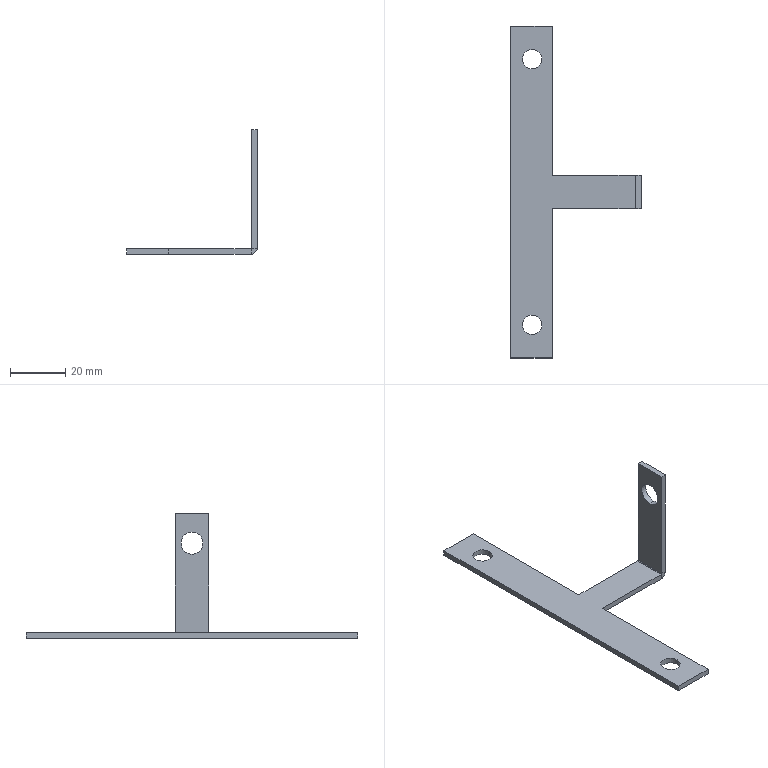Part | STEP file | Sensor bracket | 1 solid | 24 faces | box 47.2 x 120 x 45 mm | volume 5138 mm3 | plane 16 | cylinder 8 | commonest cylinder face diameters 7 x4 8 x2 0.4 x1 4.4 x1
STEP:
#1=CARTESIAN_POINT('',(39.7,0.,36.373));
#2=VERTEX_POINT('',#1);
#3=CARTESIAN_POINT('',(39.7,0.,28.373));
#4=VERTEX_POINT('',#3);
#5=CARTESIAN_POINT('',(39.7,0.,32.373));
#6=DIRECTION('',(1.,0.,0.));
#7=DIRECTION('',(0.,0.,1.));
#8=AXIS2_PLACEMENT_3D('',#5,#6,#7);
#9=CIRCLE('',#8,4.);
#10=EDGE_CURVE('',#2,#4,#9,.T.);
#11=ORIENTED_EDGE('',*,*,#10,.T.);
#12=CARTESIAN_POINT('',(37.7,0.,28.373));
#13=VERTEX_POINT('',#12);
#14=CARTESIAN_POINT('',(39.701,0.,28.373));
#15=DIRECTION('',(-1.,0.,0.));
#16=VECTOR('',#15,1000.);
#17=LINE('',#14,#16);
#18=EDGE_CURVE('',#4,#13,#17,.T.);
#19=ORIENTED_EDGE('',*,*,#18,.T.);
#20=CARTESIAN_POINT('',(37.7,0.,36.373));
#21=VERTEX_POINT('',#20);
#22=CARTESIAN_POINT('',(37.7,0.,32.373));
#23=DIRECTION('',(-1.,0.,0.));
#24=DIRECTION('',(0.,0.,1.));
#25=AXIS2_PLACEMENT_3D('',#22,#23,#24);
#26=CIRCLE('',#25,4.);
#27=EDGE_CURVE('',#13,#21,#26,.T.);
#28=ORIENTED_EDGE('',*,*,#27,.T.);
#29=CARTESIAN_POINT('',(39.701,0.,36.373));
#30=DIRECTION('',(-1.,0.,0.));
#31=VECTOR('',#30,1000.);
#32=LINE('',#29,#31);
#33=EDGE_CURVE('',#2,#21,#32,.T.);
#34=ORIENTED_EDGE('',*,*,#33,.F.);
#35=EDGE_LOOP('',(#11,#19,#28,#34));
#36=FACE_OUTER_BOUND('',#35,.T.);
#37=CARTESIAN_POINT('',(39.701,0.,32.373));
#38=DIRECTION('',(-1.,0.,0.));
#39=DIRECTION('',(0.,0.,1.));
#40=AXIS2_PLACEMENT_3D('',#37,#38,#39);
#41=CYLINDRICAL_SURFACE('',#40,4.);
#42=ADVANCED_FACE('',(#36),#41,.F.);
#43=CARTESIAN_POINT('',(-3.236,48.,-2.));
#44=VERTEX_POINT('',#43);
#45=CARTESIAN_POINT('',(3.764,48.,-2.));
#46=VERTEX_POINT('',#45);
#47=CARTESIAN_POINT('',(0.2639,48.,-2.));
#48=DIRECTION('',(0.,0.,1.));
#49=DIRECTION('',(-1.,0.,0.));
#50=AXIS2_PLACEMENT_3D('',#47,#48,#49);
#51=CIRCLE('',#50,3.5);
#52=EDGE_CURVE('',#44,#46,#51,.T.);
#53=ORIENTED_EDGE('',*,*,#52,.F.);
#54=CARTESIAN_POINT('',(-3.236,48.,0.));
#55=VERTEX_POINT('',#54);
#56=CARTESIAN_POINT('',(-3.236,48.,-2.001));
#57=DIRECTION('',(0.,0.,1.));
#58=VECTOR('',#57,1000.);
#59=LINE('',#56,#58);
#60=EDGE_CURVE('',#44,#55,#59,.T.);
#61=ORIENTED_EDGE('',*,*,#60,.T.);
#62=CARTESIAN_POINT('',(3.764,48.,0.));
#63=VERTEX_POINT('',#62);
#64=CARTESIAN_POINT('',(0.2639,48.,0.));
#65=DIRECTION('',(0.,0.,1.));
#66=DIRECTION('',(1.,0.,0.));
#67=AXIS2_PLACEMENT_3D('',#64,#65,#66);
#68=CIRCLE('',#67,3.5);
#69=EDGE_CURVE('',#55,#63,#68,.T.);
#70=ORIENTED_EDGE('',*,*,#69,.T.);
#71=CARTESIAN_POINT('',(3.764,48.,-2.001));
#72=DIRECTION('',(0.,0.,1.));
#73=VECTOR('',#72,1000.);
#74=LINE('',#71,#73);
#75=EDGE_CURVE('',#46,#63,#74,.T.);
#76=ORIENTED_EDGE('',*,*,#75,.F.);
#77=EDGE_LOOP('',(#53,#61,#70,#76));
#78=FACE_OUTER_BOUND('',#77,.T.);
#79=CARTESIAN_POINT('',(0.2639,48.,-2.001));
#80=DIRECTION('',(0.,0.,1.));
#81=DIRECTION('',(1.,0.,0.));
#82=AXIS2_PLACEMENT_3D('',#79,#80,#81);
#83=CYLINDRICAL_SURFACE('',#82,3.5);
#84=ADVANCED_FACE('',(#78),#83,.F.);
#85=CARTESIAN_POINT('',(-3.236,-48.,-2.));
#86=VERTEX_POINT('',#85);
#87=CARTESIAN_POINT('',(3.764,-48.,-2.));
#88=VERTEX_POINT('',#87);
#89=CARTESIAN_POINT('',(0.2639,-48.,-2.));
#90=DIRECTION('',(0.,0.,1.));
#91=DIRECTION('',(-1.,0.,0.));
#92=AXIS2_PLACEMENT_3D('',#89,#90,#91);
#93=CIRCLE('',#92,3.5);
#94=EDGE_CURVE('',#86,#88,#93,.T.);
#95=ORIENTED_EDGE('',*,*,#94,.F.);
#96=CARTESIAN_POINT('',(-3.236,-48.,0.));
#97=VERTEX_POINT('',#96);
#98=CARTESIAN_POINT('',(-3.236,-48.,-2.001));
#99=DIRECTION('',(0.,0.,1.));
#100=VECTOR('',#99,1000.);
#101=LINE('',#98,#100);
#102=EDGE_CURVE('',#86,#97,#101,.T.);
#103=ORIENTED_EDGE('',*,*,#102,.T.);
#104=CARTESIAN_POINT('',(3.764,-48.,0.));
#105=VERTEX_POINT('',#104);
#106=CARTESIAN_POINT('',(0.2639,-48.,0.));
#107=DIRECTION('',(0.,0.,1.));
#108=DIRECTION('',(1.,0.,0.));
#109=AXIS2_PLACEMENT_3D('',#106,#107,#108);
#110=CIRCLE('',#109,3.5);
#111=EDGE_CURVE('',#97,#105,#110,.T.);
#112=ORIENTED_EDGE('',*,*,#111,.T.);
#113=CARTESIAN_POINT('',(3.764,-48.,-2.001));
#114=DIRECTION('',(0.,0.,1.));
#115=VECTOR('',#114,1000.);
#116=LINE('',#113,#115);
#117=EDGE_CURVE('',#88,#105,#116,.T.);
#118=ORIENTED_EDGE('',*,*,#117,.F.);
#119=EDGE_LOOP('',(#95,#103,#112,#118));
#120=FACE_OUTER_BOUND('',#119,.T.);
#121=CARTESIAN_POINT('',(0.2639,-48.,-2.001));
#122=DIRECTION('',(0.,0.,1.));
#123=DIRECTION('',(1.,0.,0.));
#124=AXIS2_PLACEMENT_3D('',#121,#122,#123);
#125=CYLINDRICAL_SURFACE('',#124,3.5);
#126=ADVANCED_FACE('',(#120),#125,.F.);
#127=CARTESIAN_POINT('',(7.5,6.,0.));
#128=VERTEX_POINT('',#127);
#129=CARTESIAN_POINT('',(7.5,60.,0.));
#130=VERTEX_POINT('',#129);
#131=CARTESIAN_POINT('',(7.5,6.,0.));
#132=DIRECTION('',(0.,1.,0.));
#133=VECTOR('',#132,1000.);
#134=LINE('',#131,#133);
#135=EDGE_CURVE('',#128,#130,#134,.T.);
#136=ORIENTED_EDGE('',*,*,#135,.F.);
#137=CARTESIAN_POINT('',(7.5,6.,-2.));
#138=VERTEX_POINT('',#137);
#139=CARTESIAN_POINT('',(7.5,6.,-2.));
#140=DIRECTION('',(0.,0.,1.));
#141=VECTOR('',#140,1000.);
#142=LINE('',#139,#141);
#143=EDGE_CURVE('',#138,#128,#142,.T.);
#144=ORIENTED_EDGE('',*,*,#143,.F.);
#145=CARTESIAN_POINT('',(7.5,60.,-2.));
#146=VERTEX_POINT('',#145);
#147=CARTESIAN_POINT('',(7.5,6.,-2.));
#148=DIRECTION('',(0.,1.,0.));
#149=VECTOR('',#148,1000.);
#150=LINE('',#147,#149);
#151=EDGE_CURVE('',#138,#146,#150,.T.);
#152=ORIENTED_EDGE('',*,*,#151,.T.);
#153=CARTESIAN_POINT('',(7.5,60.,-2.));
#154=DIRECTION('',(0.,0.,1.));
#155=VECTOR('',#154,1000.);
#156=LINE('',#153,#155);
#157=EDGE_CURVE('',#146,#130,#156,.T.);
#158=ORIENTED_EDGE('',*,*,#157,.T.);
#159=EDGE_LOOP('',(#136,#144,#152,#158));
#160=FACE_OUTER_BOUND('',#159,.T.);
#161=CARTESIAN_POINT('',(7.5,6.,-2.));
#162=DIRECTION('',(1.,0.,0.));
#163=DIRECTION('',(0.,1.,0.));
#164=AXIS2_PLACEMENT_3D('',#161,#162,#163);
#165=PLANE('',#164);
#166=ADVANCED_FACE('',(#160),#165,.T.);
#167=CARTESIAN_POINT('',(37.5,6.,0.));
#168=VERTEX_POINT('',#167);
#169=CARTESIAN_POINT('',(37.5,6.,0.));
#170=DIRECTION('',(-1.,0.,0.));
#171=VECTOR('',#170,1000.);
#172=LINE('',#169,#171);
#173=EDGE_CURVE('',#168,#128,#172,.T.);
#174=ORIENTED_EDGE('',*,*,#173,.F.);
#175=CARTESIAN_POINT('',(37.5,6.,-2.));
#176=VERTEX_POINT('',#175);
#177=CARTESIAN_POINT('',(37.5,6.,-2.));
#178=DIRECTION('',(0.,0.,1.));
#179=VECTOR('',#178,1000.);
#180=LINE('',#177,#179);
#181=EDGE_CURVE('',#176,#168,#180,.T.);
#182=ORIENTED_EDGE('',*,*,#181,.F.);
#183=CARTESIAN_POINT('',(37.5,6.,-2.));
#184=DIRECTION('',(-1.,0.,0.));
#185=VECTOR('',#184,1000.);
#186=LINE('',#183,#185);
#187=EDGE_CURVE('',#176,#138,#186,.T.);
#188=ORIENTED_EDGE('',*,*,#187,.T.);
#189=ORIENTED_EDGE('',*,*,#143,.T.);
#190=EDGE_LOOP('',(#174,#182,#188,#189));
#191=FACE_OUTER_BOUND('',#190,.T.);
#192=CARTESIAN_POINT('',(37.5,6.,-2.));
#193=DIRECTION('',(0.,1.,0.));
#194=DIRECTION('',(-1.,0.,0.));
#195=AXIS2_PLACEMENT_3D('',#192,#193,#194);
#196=PLANE('',#195);
#197=ADVANCED_FACE('',(#191),#196,.T.);
#198=CARTESIAN_POINT('',(7.5,-6.,0.));
#199=VERTEX_POINT('',#198);
#200=CARTESIAN_POINT('',(37.5,-6.,0.));
#201=VERTEX_POINT('',#200);
#202=CARTESIAN_POINT('',(37.5,-6.,0.));
#203=DIRECTION('',(1.,0.,0.));
#204=VECTOR('',#203,1000.);
#205=LINE('',#202,#204);
#206=EDGE_CURVE('',#199,#201,#205,.T.);
#207=ORIENTED_EDGE('',*,*,#206,.F.);
#208=CARTESIAN_POINT('',(7.5,-6.,-2.));
#209=VERTEX_POINT('',#208);
#210=CARTESIAN_POINT('',(7.5,-6.,-2.));
#211=DIRECTION('',(0.,0.,1.));
#212=VECTOR('',#211,1000.);
#213=LINE('',#210,#212);
#214=EDGE_CURVE('',#209,#199,#213,.T.);
#215=ORIENTED_EDGE('',*,*,#214,.F.);
#216=CARTESIAN_POINT('',(37.5,-6.,-2.));
#217=VERTEX_POINT('',#216);
#218=CARTESIAN_POINT('',(37.5,-6.,-2.));
#219=DIRECTION('',(1.,0.,0.));
#220=VECTOR('',#219,1000.);
#221=LINE('',#218,#220);
#222=EDGE_CURVE('',#209,#217,#221,.T.);
#223=ORIENTED_EDGE('',*,*,#222,.T.);
#224=CARTESIAN_POINT('',(37.5,-6.,-2.));
#225=DIRECTION('',(0.,0.,1.));
#226=VECTOR('',#225,1000.);
#227=LINE('',#224,#226);
#228=EDGE_CURVE('',#217,#201,#227,.T.);
#229=ORIENTED_EDGE('',*,*,#228,.T.);
#230=EDGE_LOOP('',(#207,#215,#223,#229));
#231=FACE_OUTER_BOUND('',#230,.T.);
#232=CARTESIAN_POINT('',(37.5,-6.,-2.));
#233=DIRECTION('',(0.,-1.,0.));
#234=DIRECTION('',(1.,0.,0.));
#235=AXIS2_PLACEMENT_3D('',#232,#233,#234);
#236=PLANE('',#235);
#237=ADVANCED_FACE('',(#231),#236,.T.);
#238=CARTESIAN_POINT('',(7.5,-60.,0.));
#239=VERTEX_POINT('',#238);
#240=CARTESIAN_POINT('',(7.5,-60.,0.));
#241=DIRECTION('',(0.,1.,0.));
#242=VECTOR('',#241,1000.);
#243=LINE('',#240,#242);
#244=EDGE_CURVE('',#239,#199,#243,.T.);
#245=ORIENTED_EDGE('',*,*,#244,.F.);
#246=CARTESIAN_POINT('',(7.5,-60.,-2.));
#247=VERTEX_POINT('',#246);
#248=CARTESIAN_POINT('',(7.5,-60.,-2.));
#249=DIRECTION('',(0.,0.,1.));
#250=VECTOR('',#249,1000.);
#251=LINE('',#248,#250);
#252=EDGE_CURVE('',#247,#239,#251,.T.);
#253=ORIENTED_EDGE('',*,*,#252,.F.);
#254=CARTESIAN_POINT('',(7.5,-60.,-2.));
#255=DIRECTION('',(0.,1.,0.));
#256=VECTOR('',#255,1000.);
#257=LINE('',#254,#256);
#258=EDGE_CURVE('',#247,#209,#257,.T.);
#259=ORIENTED_EDGE('',*,*,#258,.T.);
#260=ORIENTED_EDGE('',*,*,#214,.T.);
#261=EDGE_LOOP('',(#245,#253,#259,#260));
#262=FACE_OUTER_BOUND('',#261,.T.);
#263=CARTESIAN_POINT('',(7.5,-60.,-2.));
#264=DIRECTION('',(1.,0.,0.));
#265=DIRECTION('',(0.,0.,-1.));
#266=AXIS2_PLACEMENT_3D('',#263,#264,#265);
#267=PLANE('',#266);
#268=ADVANCED_FACE('',(#262),#267,.T.);
#269=CARTESIAN_POINT('',(-7.5,-60.,0.));
#270=VERTEX_POINT('',#269);
#271=CARTESIAN_POINT('',(-7.5,-60.,0.));
#272=DIRECTION('',(1.,0.,0.));
#273=VECTOR('',#272,1000.);
#274=LINE('',#271,#273);
#275=EDGE_CURVE('',#270,#239,#274,.T.);
#276=ORIENTED_EDGE('',*,*,#275,.F.);
#277=CARTESIAN_POINT('',(-7.5,-60.,-2.));
#278=VERTEX_POINT('',#277);
#279=CARTESIAN_POINT('',(-7.5,-60.,-2.));
#280=DIRECTION('',(0.,0.,1.));
#281=VECTOR('',#280,1000.);
#282=LINE('',#279,#281);
#283=EDGE_CURVE('',#278,#270,#282,.T.);
#284=ORIENTED_EDGE('',*,*,#283,.F.);
#285=CARTESIAN_POINT('',(-7.5,-60.,-2.));
#286=DIRECTION('',(1.,0.,0.));
#287=VECTOR('',#286,1000.);
#288=LINE('',#285,#287);
#289=EDGE_CURVE('',#278,#247,#288,.T.);
#290=ORIENTED_EDGE('',*,*,#289,.T.);
#291=ORIENTED_EDGE('',*,*,#252,.T.);
#292=EDGE_LOOP('',(#276,#284,#290,#291));
#293=FACE_OUTER_BOUND('',#292,.T.);
#294=CARTESIAN_POINT('',(-7.5,-60.,-2.));
#295=DIRECTION('',(0.,-1.,0.));
#296=DIRECTION('',(0.,0.,-1.));
#297=AXIS2_PLACEMENT_3D('',#294,#295,#296);
#298=PLANE('',#297);
#299=ADVANCED_FACE('',(#293),#298,.T.);
#300=CARTESIAN_POINT('',(-7.5,60.,0.));
#301=VERTEX_POINT('',#300);
#302=CARTESIAN_POINT('',(-7.5,-60.,0.));
#303=DIRECTION('',(0.,-1.,0.));
#304=VECTOR('',#303,1000.);
#305=LINE('',#302,#304);
#306=EDGE_CURVE('',#301,#270,#305,.T.);
#307=ORIENTED_EDGE('',*,*,#306,.F.);
#308=CARTESIAN_POINT('',(-7.5,60.,-2.));
#309=VERTEX_POINT('',#308);
#310=CARTESIAN_POINT('',(-7.5,60.,-2.));
#311=DIRECTION('',(0.,0.,1.));
#312=VECTOR('',#311,1000.);
#313=LINE('',#310,#312);
#314=EDGE_CURVE('',#309,#301,#313,.T.);
#315=ORIENTED_EDGE('',*,*,#314,.F.);
#316=CARTESIAN_POINT('',(-7.5,-60.,-2.));
#317=DIRECTION('',(0.,-1.,0.));
#318=VECTOR('',#317,1000.);
#319=LINE('',#316,#318);
#320=EDGE_CURVE('',#309,#278,#319,.T.);
#321=ORIENTED_EDGE('',*,*,#320,.T.);
#322=ORIENTED_EDGE('',*,*,#283,.T.);
#323=EDGE_LOOP('',(#307,#315,#321,#322));
#324=FACE_OUTER_BOUND('',#323,.T.);
#325=CARTESIAN_POINT('',(-7.5,-60.,-2.));
#326=DIRECTION('',(-1.,0.,0.));
#327=DIRECTION('',(0.,0.,1.));
#328=AXIS2_PLACEMENT_3D('',#325,#326,#327);
#329=PLANE('',#328);
#330=ADVANCED_FACE('',(#324),#329,.T.);
#331=CARTESIAN_POINT('',(-7.5,60.,0.));
#332=DIRECTION('',(-1.,0.,0.));
#333=VECTOR('',#332,1000.);
#334=LINE('',#331,#333);
#335=EDGE_CURVE('',#130,#301,#334,.T.);
#336=ORIENTED_EDGE('',*,*,#335,.F.);
#337=ORIENTED_EDGE('',*,*,#157,.F.);
#338=CARTESIAN_POINT('',(-7.5,60.,-2.));
#339=DIRECTION('',(-1.,0.,0.));
#340=VECTOR('',#339,1000.);
#341=LINE('',#338,#340);
#342=EDGE_CURVE('',#146,#309,#341,.T.);
#343=ORIENTED_EDGE('',*,*,#342,.T.);
#344=ORIENTED_EDGE('',*,*,#314,.T.);
#345=EDGE_LOOP('',(#336,#337,#343,#344));
#346=FACE_OUTER_BOUND('',#345,.T.);
#347=CARTESIAN_POINT('',(-7.5,60.,-2.));
#348=DIRECTION('',(0.,1.,0.));
#349=DIRECTION('',(0.,0.,1.));
#350=AXIS2_PLACEMENT_3D('',#347,#348,#349);
#351=PLANE('',#350);
#352=ADVANCED_FACE('',(#346),#351,.T.);
#353=CARTESIAN_POINT('',(0.2639,48.,-2.));
#354=DIRECTION('',(0.,0.,1.));
#355=DIRECTION('',(-1.,0.,0.));
#356=AXIS2_PLACEMENT_3D('',#353,#354,#355);
#357=CIRCLE('',#356,3.5);
#358=EDGE_CURVE('',#46,#44,#357,.T.);
#359=ORIENTED_EDGE('',*,*,#358,.T.);
#360=ORIENTED_EDGE('',*,*,#52,.T.);
#361=EDGE_LOOP('',(#359,#360));
#362=FACE_BOUND('',#361,.T.);
#363=CARTESIAN_POINT('',(0.2639,-48.,-2.));
#364=DIRECTION('',(0.,0.,1.));
#365=DIRECTION('',(-1.,0.,0.));
#366=AXIS2_PLACEMENT_3D('',#363,#364,#365);
#367=CIRCLE('',#366,3.5);
#368=EDGE_CURVE('',#88,#86,#367,.T.);
#369=ORIENTED_EDGE('',*,*,#368,.T.);
#370=ORIENTED_EDGE('',*,*,#94,.T.);
#371=EDGE_LOOP('',(#369,#370));
#372=FACE_BOUND('',#371,.T.);
#373=ORIENTED_EDGE('',*,*,#151,.F.);
#374=ORIENTED_EDGE('',*,*,#187,.F.);
#375=CARTESIAN_POINT('',(37.5,-6.,-2.));
#376=DIRECTION('',(0.,1.,0.));
#377=VECTOR('',#376,1000.);
#378=LINE('',#375,#377);
#379=EDGE_CURVE('',#217,#176,#378,.T.);
#380=ORIENTED_EDGE('',*,*,#379,.F.);
#381=ORIENTED_EDGE('',*,*,#222,.F.);
#382=ORIENTED_EDGE('',*,*,#258,.F.);
#383=ORIENTED_EDGE('',*,*,#289,.F.);
#384=ORIENTED_EDGE('',*,*,#320,.F.);
#385=ORIENTED_EDGE('',*,*,#342,.F.);
#386=EDGE_LOOP('',(#373,#374,#380,#381,#382,#383,#384,#385));
#387=FACE_OUTER_BOUND('',#386,.T.);
#388=CARTESIAN_POINT('',(0.,0.,-2.));
#389=DIRECTION('',(0.,0.,-1.));
#390=DIRECTION('',(-1.,0.,0.));
#391=AXIS2_PLACEMENT_3D('',#388,#389,#390);
#392=PLANE('',#391);
#393=ADVANCED_FACE('',(#362,#372,#387),#392,.T.);
#394=CARTESIAN_POINT('',(0.2639,48.,0.));
#395=DIRECTION('',(0.,0.,1.));
#396=DIRECTION('',(1.,0.,0.));
#397=AXIS2_PLACEMENT_3D('',#394,#395,#396);
#398=CIRCLE('',#397,3.5);
#399=EDGE_CURVE('',#63,#55,#398,.T.);
#400=ORIENTED_EDGE('',*,*,#399,.F.);
#401=ORIENTED_EDGE('',*,*,#69,.F.);
#402=EDGE_LOOP('',(#400,#401));
#403=FACE_BOUND('',#402,.T.);
#404=CARTESIAN_POINT('',(0.2639,-48.,0.));
#405=DIRECTION('',(0.,0.,1.));
#406=DIRECTION('',(1.,0.,0.));
#407=AXIS2_PLACEMENT_3D('',#404,#405,#406);
#408=CIRCLE('',#407,3.5);
#409=EDGE_CURVE('',#105,#97,#408,.T.);
#410=ORIENTED_EDGE('',*,*,#409,.F.);
#411=ORIENTED_EDGE('',*,*,#111,.F.);
#412=EDGE_LOOP('',(#410,#411));
#413=FACE_BOUND('',#412,.T.);
#414=ORIENTED_EDGE('',*,*,#135,.T.);
#415=ORIENTED_EDGE('',*,*,#335,.T.);
#416=ORIENTED_EDGE('',*,*,#306,.T.);
#417=ORIENTED_EDGE('',*,*,#275,.T.);
#418=ORIENTED_EDGE('',*,*,#244,.T.);
#419=ORIENTED_EDGE('',*,*,#206,.T.);
#420=CARTESIAN_POINT('',(37.5,-6.,0.));
#421=DIRECTION('',(0.,1.,0.));
#422=VECTOR('',#421,1000.);
#423=LINE('',#420,#422);
#424=EDGE_CURVE('',#201,#168,#423,.T.);
#425=ORIENTED_EDGE('',*,*,#424,.T.);
#426=ORIENTED_EDGE('',*,*,#173,.T.);
#427=EDGE_LOOP('',(#414,#415,#416,#417,#418,#419,#425,#426));
#428=FACE_OUTER_BOUND('',#427,.T.);
#429=CARTESIAN_POINT('',(0.,0.,0.));
#430=DIRECTION('',(0.,0.,-1.));
#431=DIRECTION('',(-1.,0.,0.));
#432=AXIS2_PLACEMENT_3D('',#429,#430,#431);
#433=PLANE('',#432);
#434=ADVANCED_FACE('',(#403,#413,#428),#433,.F.);
#435=ORIENTED_EDGE('',*,*,#102,.F.);
#436=ORIENTED_EDGE('',*,*,#368,.F.);
#437=ORIENTED_EDGE('',*,*,#117,.T.);
#438=ORIENTED_EDGE('',*,*,#409,.T.);
#439=EDGE_LOOP('',(#435,#436,#437,#438));
#440=FACE_OUTER_BOUND('',#439,.T.);
#441=CARTESIAN_POINT('',(0.2639,-48.,-2.001));
#442=DIRECTION('',(0.,0.,1.));
#443=DIRECTION('',(1.,0.,0.));
#444=AXIS2_PLACEMENT_3D('',#441,#442,#443);
#445=CYLINDRICAL_SURFACE('',#444,3.5);
#446=ADVANCED_FACE('',(#440),#445,.F.);
#447=ORIENTED_EDGE('',*,*,#60,.F.);
#448=ORIENTED_EDGE('',*,*,#358,.F.);
#449=ORIENTED_EDGE('',*,*,#75,.T.);
#450=ORIENTED_EDGE('',*,*,#399,.T.);
#451=EDGE_LOOP('',(#447,#448,#449,#450));
#452=FACE_OUTER_BOUND('',#451,.T.);
#453=CARTESIAN_POINT('',(0.2639,48.,-2.001));
#454=DIRECTION('',(0.,0.,1.));
#455=DIRECTION('',(1.,0.,0.));
#456=AXIS2_PLACEMENT_3D('',#453,#454,#455);
#457=CYLINDRICAL_SURFACE('',#456,3.5);
#458=ADVANCED_FACE('',(#452),#457,.F.);
#459=CARTESIAN_POINT('',(37.7,-6.,0.2));
#460=VERTEX_POINT('',#459);
#461=CARTESIAN_POINT('',(39.7,-6.,0.2));
#462=VERTEX_POINT('',#461);
#463=CARTESIAN_POINT('',(39.7,-6.,0.2));
#464=DIRECTION('',(1.,0.,0.));
#465=VECTOR('',#464,1000.);
#466=LINE('',#463,#465);
#467=EDGE_CURVE('',#460,#462,#466,.T.);
#468=ORIENTED_EDGE('',*,*,#467,.F.);
#469=CARTESIAN_POINT('',(37.5,-6.,0.2));
#470=DIRECTION('',(0.,-1.,0.));
#471=DIRECTION('',(0.,0.,1.));
#472=AXIS2_PLACEMENT_3D('',#469,#470,#471);
#473=CIRCLE('',#472,0.2);
#474=EDGE_CURVE('',#201,#460,#473,.T.);
#475=ORIENTED_EDGE('',*,*,#474,.F.);
#476=ORIENTED_EDGE('',*,*,#228,.F.);
#477=CARTESIAN_POINT('',(37.5,-6.,0.2));
#478=DIRECTION('',(0.,-1.,0.));
#479=DIRECTION('',(0.,0.,1.));
#480=AXIS2_PLACEMENT_3D('',#477,#478,#479);
#481=CIRCLE('',#480,2.2);
#482=EDGE_CURVE('',#217,#462,#481,.T.);
#483=ORIENTED_EDGE('',*,*,#482,.T.);
#484=EDGE_LOOP('',(#468,#475,#476,#483));
#485=FACE_OUTER_BOUND('',#484,.T.);
#486=CARTESIAN_POINT('',(37.5,-6.,0.2));
#487=DIRECTION('',(0.,-1.,0.));
#488=DIRECTION('',(0.,0.,-1.));
#489=AXIS2_PLACEMENT_3D('',#486,#487,#488);
#490=PLANE('',#489);
#491=ADVANCED_FACE('',(#485),#490,.T.);
#492=CARTESIAN_POINT('',(37.7,6.,0.2));
#493=VERTEX_POINT('',#492);
#494=CARTESIAN_POINT('',(37.5,6.,0.2));
#495=DIRECTION('',(0.,1.,0.));
#496=DIRECTION('',(0.,0.,1.));
#497=AXIS2_PLACEMENT_3D('',#494,#495,#496);
#498=CIRCLE('',#497,0.2);
#499=EDGE_CURVE('',#493,#168,#498,.T.);
#500=ORIENTED_EDGE('',*,*,#499,.F.);
#501=CARTESIAN_POINT('',(39.7,6.,0.2));
#502=VERTEX_POINT('',#501);
#503=CARTESIAN_POINT('',(37.7,6.,0.2));
#504=DIRECTION('',(1.,0.,0.));
#505=VECTOR('',#504,1000.);
#506=LINE('',#503,#505);
#507=EDGE_CURVE('',#493,#502,#506,.T.);
#508=ORIENTED_EDGE('',*,*,#507,.T.);
#509=CARTESIAN_POINT('',(37.5,6.,0.2));
#510=DIRECTION('',(0.,1.,0.));
#511=DIRECTION('',(0.,0.,1.));
#512=AXIS2_PLACEMENT_3D('',#509,#510,#511);
#513=CIRCLE('',#512,2.2);
#514=EDGE_CURVE('',#502,#176,#513,.T.);
#515=ORIENTED_EDGE('',*,*,#514,.T.);
#516=ORIENTED_EDGE('',*,*,#181,.T.);
#517=EDGE_LOOP('',(#500,#508,#515,#516));
#518=FACE_OUTER_BOUND('',#517,.T.);
#519=CARTESIAN_POINT('',(37.5,6.,0.2));
#520=DIRECTION('',(0.,-1.,0.));
#521=DIRECTION('',(0.,0.,-1.));
#522=AXIS2_PLACEMENT_3D('',#519,#520,#521);
#523=PLANE('',#522);
#524=ADVANCED_FACE('',(#518),#523,.F.);
#525=ORIENTED_EDGE('',*,*,#379,.T.);
#526=ORIENTED_EDGE('',*,*,#514,.F.);
#527=CARTESIAN_POINT('',(39.7,-6.,0.2));
#528=DIRECTION('',(0.,-1.,0.));
#529=VECTOR('',#528,1000.);
#530=LINE('',#527,#529);
#531=EDGE_CURVE('',#502,#462,#530,.T.);
#532=ORIENTED_EDGE('',*,*,#531,.T.);
#533=ORIENTED_EDGE('',*,*,#482,.F.);
#534=EDGE_LOOP('',(#525,#526,#532,#533));
#535=FACE_OUTER_BOUND('',#534,.T.);
#536=CARTESIAN_POINT('',(37.5,6.,0.2));
#537=DIRECTION('',(0.,1.,0.));
#538=DIRECTION('',(1.,0.,0.));
#539=AXIS2_PLACEMENT_3D('',#536,#537,#538);
#540=CYLINDRICAL_SURFACE('',#539,2.2);
#541=ADVANCED_FACE('',(#535),#540,.T.);
#542=ORIENTED_EDGE('',*,*,#424,.F.);
#543=ORIENTED_EDGE('',*,*,#474,.T.);
#544=CARTESIAN_POINT('',(37.7,-6.,0.2));
#545=DIRECTION('',(0.,1.,0.));
#546=VECTOR('',#545,1000.);
#547=LINE('',#544,#546);
#548=EDGE_CURVE('',#460,#493,#547,.T.);
#549=ORIENTED_EDGE('',*,*,#548,.T.);
#550=ORIENTED_EDGE('',*,*,#499,.T.);
#551=EDGE_LOOP('',(#542,#543,#549,#550));
#552=FACE_OUTER_BOUND('',#551,.T.);
#553=CARTESIAN_POINT('',(37.5,6.,0.2));
#554=DIRECTION('',(0.,1.,0.));
#555=DIRECTION('',(1.,0.,0.));
#556=AXIS2_PLACEMENT_3D('',#553,#554,#555);
#557=CYLINDRICAL_SURFACE('',#556,0.2);
#558=ADVANCED_FACE('',(#552),#557,.F.);
#559=ORIENTED_EDGE('',*,*,#467,.T.);
#560=CARTESIAN_POINT('',(39.7,-6.,43.));
#561=VERTEX_POINT('',#560);
#562=CARTESIAN_POINT('',(39.7,-6.,0.));
#563=DIRECTION('',(0.,0.,-1.));
#564=VECTOR('',#563,1000.);
#565=LINE('',#562,#564);
#566=EDGE_CURVE('',#561,#462,#565,.T.);
#567=ORIENTED_EDGE('',*,*,#566,.F.);
#568=CARTESIAN_POINT('',(37.7,-6.,43.));
#569=VERTEX_POINT('',#568);
#570=CARTESIAN_POINT('',(39.7,-6.,43.));
#571=DIRECTION('',(-1.,0.,0.));
#572=VECTOR('',#571,1000.);
#573=LINE('',#570,#572);
#574=EDGE_CURVE('',#561,#569,#573,.T.);
#575=ORIENTED_EDGE('',*,*,#574,.T.);
#576=CARTESIAN_POINT('',(37.7,-6.,0.));
#577=DIRECTION('',(0.,0.,-1.));
#578=VECTOR('',#577,1000.);
#579=LINE('',#576,#578);
#580=EDGE_CURVE('',#569,#460,#579,.T.);
#581=ORIENTED_EDGE('',*,*,#580,.T.);
#582=EDGE_LOOP('',(#559,#567,#575,#581));
#583=FACE_OUTER_BOUND('',#582,.T.);
#584=CARTESIAN_POINT('',(39.7,-6.,0.));
#585=DIRECTION('',(0.,1.,0.));
#586=DIRECTION('',(0.,0.,1.));
#587=AXIS2_PLACEMENT_3D('',#584,#585,#586);
#588=PLANE('',#587);
#589=ADVANCED_FACE('',(#583),#588,.F.);
#590=ORIENTED_EDGE('',*,*,#507,.F.);
#591=CARTESIAN_POINT('',(37.7,6.,43.));
#592=VERTEX_POINT('',#591);
#593=CARTESIAN_POINT('',(37.7,6.,43.));
#594=DIRECTION('',(0.,0.,1.));
#595=VECTOR('',#594,1000.);
#596=LINE('',#593,#595);
#597=EDGE_CURVE('',#493,#592,#596,.T.);
#598=ORIENTED_EDGE('',*,*,#597,.T.);
#599=CARTESIAN_POINT('',(39.7,6.,43.));
#600=VERTEX_POINT('',#599);
#601=CARTESIAN_POINT('',(39.7,6.,43.));
#602=DIRECTION('',(-1.,0.,0.));
#603=VECTOR('',#602,1000.);
#604=LINE('',#601,#603);
#605=EDGE_CURVE('',#600,#592,#604,.T.);
#606=ORIENTED_EDGE('',*,*,#605,.F.);
#607=CARTESIAN_POINT('',(39.7,6.,0.));
#608=DIRECTION('',(0.,0.,1.));
#609=VECTOR('',#608,1000.);
#610=LINE('',#607,#609);
#611=EDGE_CURVE('',#502,#600,#610,.T.);
#612=ORIENTED_EDGE('',*,*,#611,.F.);
#613=EDGE_LOOP('',(#590,#598,#606,#612));
#614=FACE_OUTER_BOUND('',#613,.T.);
#615=CARTESIAN_POINT('',(39.7,6.,43.));
#616=DIRECTION('',(0.,-1.,0.));
#617=DIRECTION('',(0.,0.,-1.));
#618=AXIS2_PLACEMENT_3D('',#615,#616,#617);
#619=PLANE('',#618);
#620=ADVANCED_FACE('',(#614),#619,.F.);
#621=ORIENTED_EDGE('',*,*,#10,.F.);
#622=CARTESIAN_POINT('',(39.7,0.,32.373));
#623=DIRECTION('',(1.,0.,0.));
#624=DIRECTION('',(0.,0.,1.));
#625=AXIS2_PLACEMENT_3D('',#622,#623,#624);
#626=CIRCLE('',#625,4.);
#627=EDGE_CURVE('',#4,#2,#626,.T.);
#628=ORIENTED_EDGE('',*,*,#627,.F.);
#629=EDGE_LOOP('',(#621,#628));
#630=FACE_BOUND('',#629,.T.);
#631=ORIENTED_EDGE('',*,*,#531,.F.);
#632=ORIENTED_EDGE('',*,*,#611,.T.);
#633=CARTESIAN_POINT('',(39.7,0.,43.));
#634=DIRECTION('',(0.,-1.,0.));
#635=VECTOR('',#634,1000.);
#636=LINE('',#633,#635);
#637=EDGE_CURVE('',#600,#561,#636,.T.);
#638=ORIENTED_EDGE('',*,*,#637,.T.);
#639=ORIENTED_EDGE('',*,*,#566,.T.);
#640=EDGE_LOOP('',(#631,#632,#638,#639));
#641=FACE_OUTER_BOUND('',#640,.T.);
#642=CARTESIAN_POINT('',(39.7,0.,0.));
#643=DIRECTION('',(-1.,0.,0.));
#644=DIRECTION('',(0.,0.,1.));
#645=AXIS2_PLACEMENT_3D('',#642,#643,#644);
#646=PLANE('',#645);
#647=ADVANCED_FACE('',(#630,#641),#646,.F.);
#648=CARTESIAN_POINT('',(37.7,0.,32.373));
#649=DIRECTION('',(-1.,0.,0.));
#650=DIRECTION('',(0.,0.,1.));
#651=AXIS2_PLACEMENT_3D('',#648,#649,#650);
#652=CIRCLE('',#651,4.);
#653=EDGE_CURVE('',#21,#13,#652,.T.);
#654=ORIENTED_EDGE('',*,*,#653,.F.);
#655=ORIENTED_EDGE('',*,*,#27,.F.);
#656=EDGE_LOOP('',(#654,#655));
#657=FACE_BOUND('',#656,.T.);
#658=ORIENTED_EDGE('',*,*,#597,.F.);
#659=ORIENTED_EDGE('',*,*,#548,.F.);
#660=ORIENTED_EDGE('',*,*,#580,.F.);
#661=CARTESIAN_POINT('',(37.7,-6.,43.));
#662=DIRECTION('',(0.,-1.,0.));
#663=VECTOR('',#662,1000.);
#664=LINE('',#661,#663);
#665=EDGE_CURVE('',#592,#569,#664,.T.);
#666=ORIENTED_EDGE('',*,*,#665,.F.);
#667=EDGE_LOOP('',(#658,#659,#660,#666));
#668=FACE_OUTER_BOUND('',#667,.T.);
#669=CARTESIAN_POINT('',(37.7,0.,0.));
#670=DIRECTION('',(-1.,0.,0.));
#671=DIRECTION('',(0.,0.,1.));
#672=AXIS2_PLACEMENT_3D('',#669,#670,#671);
#673=PLANE('',#672);
#674=ADVANCED_FACE('',(#657,#668),#673,.T.);
#675=ORIENTED_EDGE('',*,*,#665,.T.);
#676=ORIENTED_EDGE('',*,*,#574,.F.);
#677=ORIENTED_EDGE('',*,*,#637,.F.);
#678=ORIENTED_EDGE('',*,*,#605,.T.);
#679=EDGE_LOOP('',(#675,#676,#677,#678));
#680=FACE_OUTER_BOUND('',#679,.T.);
#681=CARTESIAN_POINT('',(39.7,-6.,43.));
#682=DIRECTION('',(0.,0.,-1.));
#683=DIRECTION('',(-1.,0.,0.));
#684=AXIS2_PLACEMENT_3D('',#681,#682,#683);
#685=PLANE('',#684);
#686=ADVANCED_FACE('',(#680),#685,.F.);
#687=ORIENTED_EDGE('',*,*,#18,.F.);
#688=ORIENTED_EDGE('',*,*,#627,.T.);
#689=ORIENTED_EDGE('',*,*,#33,.T.);
#690=ORIENTED_EDGE('',*,*,#653,.T.);
#691=EDGE_LOOP('',(#687,#688,#689,#690));
#692=FACE_OUTER_BOUND('',#691,.T.);
#693=CARTESIAN_POINT('',(39.701,0.,32.373));
#694=DIRECTION('',(-1.,0.,0.));
#695=DIRECTION('',(0.,0.,1.));
#696=AXIS2_PLACEMENT_3D('',#693,#694,#695);
#697=CYLINDRICAL_SURFACE('',#696,4.);
#698=ADVANCED_FACE('',(#692),#697,.F.);
#699=CLOSED_SHELL('',(#42,#84,#126,#166,#197,#237,#268,#299,#330,#352,#393,#434,#446,#458,#491,#524,#541,#558,#589,#620,#647,#674,#686,#698));
#700=MANIFOLD_SOLID_BREP('',#699);
#701=CARTESIAN_POINT('',(0.,0.,0.));
#702=DIRECTION('',(0.,0.,1.));
#703=DIRECTION('',(1.,0.,0.));
#704=AXIS2_PLACEMENT_3D('',#701,#702,#703);
#705=(LENGTH_UNIT()NAMED_UNIT(*)SI_UNIT(.MILLI.,.METRE.));
#706=UNCERTAINTY_MEASURE_WITH_UNIT(LENGTH_MEASURE(0.00001),#705,'','');
#707=(NAMED_UNIT(*)PLANE_ANGLE_UNIT()SI_UNIT($,.RADIAN.));
#708=(NAMED_UNIT(*)SI_UNIT($,.STERADIAN.)SOLID_ANGLE_UNIT());
#709=(GEOMETRIC_REPRESENTATION_CONTEXT(3)GLOBAL_UNCERTAINTY_ASSIGNED_CONTEXT((#706))GLOBAL_UNIT_ASSIGNED_CONTEXT((#705,#707,#708))REPRESENTATION_CONTEXT('',''));
#710=ADVANCED_BREP_SHAPE_REPRESENTATION('',(#700,#704),#709);